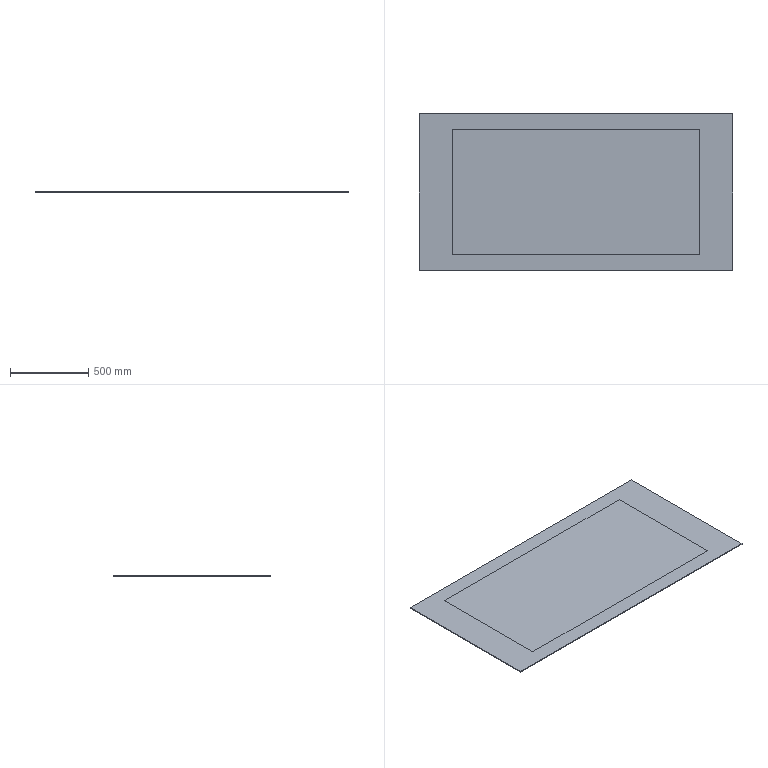Part | SolidWorks | features BaseBody 2 | 2 solids | 12 faces | box 2000 x 1000 x 5 mm | volume 16320000 mm3 | plane 12
STEP:
#1=CARTESIAN_POINT('',(-1000.,-500.,0.));
#2=VERTEX_POINT('',#1);
#3=CARTESIAN_POINT('',(1000.,-500.,0.));
#4=VERTEX_POINT('',#3);
#5=CARTESIAN_POINT('',(0.,-500.,0.));
#6=DIRECTION('',(1.,0.,0.));
#7=VECTOR('',#6,1000.);
#8=LINE('',#5,#7);
#9=EDGE_CURVE('',#2,#4,#8,.T.);
#10=ORIENTED_EDGE('',*,*,#9,.F.);
#11=CARTESIAN_POINT('',(-1000.,500.,0.));
#12=VERTEX_POINT('',#11);
#13=CARTESIAN_POINT('',(-1000.,0.,0.));
#14=DIRECTION('',(0.,-1.,0.));
#15=VECTOR('',#14,1000.);
#16=LINE('',#13,#15);
#17=EDGE_CURVE('',#12,#2,#16,.T.);
#18=ORIENTED_EDGE('',*,*,#17,.F.);
#19=CARTESIAN_POINT('',(1000.,500.,0.));
#20=VERTEX_POINT('',#19);
#21=CARTESIAN_POINT('',(0.,500.,0.));
#22=DIRECTION('',(-1.,0.,0.));
#23=VECTOR('',#22,1000.);
#24=LINE('',#21,#23);
#25=EDGE_CURVE('',#20,#12,#24,.T.);
#26=ORIENTED_EDGE('',*,*,#25,.F.);
#27=CARTESIAN_POINT('',(1000.,0.,0.));
#28=DIRECTION('',(0.,1.,0.));
#29=VECTOR('',#28,1000.);
#30=LINE('',#27,#29);
#31=EDGE_CURVE('',#4,#20,#30,.T.);
#32=ORIENTED_EDGE('',*,*,#31,.F.);
#33=EDGE_LOOP('',(#10,#18,#26,#32));
#34=FACE_OUTER_BOUND('',#33,.T.);
#35=CARTESIAN_POINT('',(0.,0.,0.));
#36=DIRECTION('',(0.,0.,1.));
#37=DIRECTION('',(1.,0.,0.));
#38=AXIS2_PLACEMENT_3D('',#35,#36,#37);
#39=PLANE('',#38);
#40=ADVANCED_FACE('',(#34),#39,.F.);
#41=ORIENTED_EDGE('',*,*,#31,.T.);
#42=CARTESIAN_POINT('',(1000.,500.,5.));
#43=VERTEX_POINT('',#42);
#44=CARTESIAN_POINT('',(1000.,500.,0.));
#45=DIRECTION('',(0.,0.,1.));
#46=VECTOR('',#45,1000.);
#47=LINE('',#44,#46);
#48=EDGE_CURVE('',#20,#43,#47,.T.);
#49=ORIENTED_EDGE('',*,*,#48,.T.);
#50=CARTESIAN_POINT('',(1000.,-500.,5.));
#51=VERTEX_POINT('',#50);
#52=CARTESIAN_POINT('',(1000.,500.,5.));
#53=DIRECTION('',(0.,-1.,0.));
#54=VECTOR('',#53,1000.);
#55=LINE('',#52,#54);
#56=EDGE_CURVE('',#43,#51,#55,.T.);
#57=ORIENTED_EDGE('',*,*,#56,.T.);
#58=CARTESIAN_POINT('',(1000.,-500.,0.));
#59=DIRECTION('',(0.,0.,-1.));
#60=VECTOR('',#59,1000.);
#61=LINE('',#58,#60);
#62=EDGE_CURVE('',#51,#4,#61,.T.);
#63=ORIENTED_EDGE('',*,*,#62,.T.);
#64=EDGE_LOOP('',(#41,#49,#57,#63));
#65=FACE_OUTER_BOUND('',#64,.T.);
#66=CARTESIAN_POINT('',(1000.,500.,0.));
#67=DIRECTION('',(1.,0.,0.));
#68=DIRECTION('',(0.,0.,-1.));
#69=AXIS2_PLACEMENT_3D('',#66,#67,#68);
#70=PLANE('',#69);
#71=ADVANCED_FACE('',(#65),#70,.T.);
#72=ORIENTED_EDGE('',*,*,#9,.T.);
#73=ORIENTED_EDGE('',*,*,#62,.F.);
#74=CARTESIAN_POINT('',(-1000.,-500.,5.));
#75=VERTEX_POINT('',#74);
#76=CARTESIAN_POINT('',(-1000.,-500.,5.));
#77=DIRECTION('',(-1.,0.,0.));
#78=VECTOR('',#77,1000.);
#79=LINE('',#76,#78);
#80=EDGE_CURVE('',#51,#75,#79,.T.);
#81=ORIENTED_EDGE('',*,*,#80,.T.);
#82=CARTESIAN_POINT('',(-1000.,-500.,0.));
#83=DIRECTION('',(0.,0.,-1.));
#84=VECTOR('',#83,1000.);
#85=LINE('',#82,#84);
#86=EDGE_CURVE('',#75,#2,#85,.T.);
#87=ORIENTED_EDGE('',*,*,#86,.T.);
#88=EDGE_LOOP('',(#72,#73,#81,#87));
#89=FACE_OUTER_BOUND('',#88,.T.);
#90=CARTESIAN_POINT('',(-1000.,-500.,0.));
#91=DIRECTION('',(0.,-1.,0.));
#92=DIRECTION('',(0.,0.,-1.));
#93=AXIS2_PLACEMENT_3D('',#90,#91,#92);
#94=PLANE('',#93);
#95=ADVANCED_FACE('',(#89),#94,.T.);
#96=ORIENTED_EDGE('',*,*,#17,.T.);
#97=ORIENTED_EDGE('',*,*,#86,.F.);
#98=CARTESIAN_POINT('',(-1000.,500.,5.));
#99=VERTEX_POINT('',#98);
#100=CARTESIAN_POINT('',(-1000.,500.,5.));
#101=DIRECTION('',(0.,1.,0.));
#102=VECTOR('',#101,1000.);
#103=LINE('',#100,#102);
#104=EDGE_CURVE('',#75,#99,#103,.T.);
#105=ORIENTED_EDGE('',*,*,#104,.T.);
#106=CARTESIAN_POINT('',(-1000.,500.,0.));
#107=DIRECTION('',(0.,0.,-1.));
#108=VECTOR('',#107,1000.);
#109=LINE('',#106,#108);
#110=EDGE_CURVE('',#99,#12,#109,.T.);
#111=ORIENTED_EDGE('',*,*,#110,.T.);
#112=EDGE_LOOP('',(#96,#97,#105,#111));
#113=FACE_OUTER_BOUND('',#112,.T.);
#114=CARTESIAN_POINT('',(-1000.,500.,0.));
#115=DIRECTION('',(-1.,0.,0.));
#116=DIRECTION('',(0.,-1.,0.));
#117=AXIS2_PLACEMENT_3D('',#114,#115,#116);
#118=PLANE('',#117);
#119=ADVANCED_FACE('',(#113),#118,.T.);
#120=ORIENTED_EDGE('',*,*,#25,.T.);
#121=ORIENTED_EDGE('',*,*,#110,.F.);
#122=CARTESIAN_POINT('',(-1000.,500.,5.));
#123=DIRECTION('',(1.,0.,0.));
#124=VECTOR('',#123,1000.);
#125=LINE('',#122,#124);
#126=EDGE_CURVE('',#99,#43,#125,.T.);
#127=ORIENTED_EDGE('',*,*,#126,.T.);
#128=ORIENTED_EDGE('',*,*,#48,.F.);
#129=EDGE_LOOP('',(#120,#121,#127,#128));
#130=FACE_OUTER_BOUND('',#129,.T.);
#131=CARTESIAN_POINT('',(-1000.,500.,0.));
#132=DIRECTION('',(0.,1.,0.));
#133=DIRECTION('',(0.,0.,1.));
#134=AXIS2_PLACEMENT_3D('',#131,#132,#133);
#135=PLANE('',#134);
#136=ADVANCED_FACE('',(#130),#135,.T.);
#137=ORIENTED_EDGE('',*,*,#104,.F.);
#138=ORIENTED_EDGE('',*,*,#80,.F.);
#139=ORIENTED_EDGE('',*,*,#56,.F.);
#140=ORIENTED_EDGE('',*,*,#126,.F.);
#141=EDGE_LOOP('',(#137,#138,#139,#140));
#142=FACE_OUTER_BOUND('',#141,.T.);
#143=CARTESIAN_POINT('',(0.,0.,5.));
#144=DIRECTION('',(0.,0.,1.));
#145=DIRECTION('',(1.,0.,0.));
#146=AXIS2_PLACEMENT_3D('',#143,#144,#145);
#147=PLANE('',#146);
#148=ADVANCED_FACE('',(#142),#147,.T.);
#149=CLOSED_SHELL('',(#40,#71,#95,#119,#136,#148));
#150=MANIFOLD_SOLID_BREP('',#149);
#151=CARTESIAN_POINT('',(-790.,400.,5.));
#152=VERTEX_POINT('',#151);
#153=CARTESIAN_POINT('',(-790.,-400.,5.));
#154=VERTEX_POINT('',#153);
#155=CARTESIAN_POINT('',(-790.,0.,5.));
#156=DIRECTION('',(0.,-1.,0.));
#157=VECTOR('',#156,1000.);
#158=LINE('',#155,#157);
#159=EDGE_CURVE('',#152,#154,#158,.T.);
#160=ORIENTED_EDGE('',*,*,#159,.T.);
#161=CARTESIAN_POINT('',(790.,-400.,5.));
#162=VERTEX_POINT('',#161);
#163=CARTESIAN_POINT('',(0.,-400.,5.));
#164=DIRECTION('',(1.,0.,0.));
#165=VECTOR('',#164,1000.);
#166=LINE('',#163,#165);
#167=EDGE_CURVE('',#154,#162,#166,.T.);
#168=ORIENTED_EDGE('',*,*,#167,.T.);
#169=CARTESIAN_POINT('',(790.,400.,5.));
#170=VERTEX_POINT('',#169);
#171=CARTESIAN_POINT('',(790.,0.,5.));
#172=DIRECTION('',(0.,1.,0.));
#173=VECTOR('',#172,1000.);
#174=LINE('',#171,#173);
#175=EDGE_CURVE('',#162,#170,#174,.T.);
#176=ORIENTED_EDGE('',*,*,#175,.T.);
#177=CARTESIAN_POINT('',(0.,400.,5.));
#178=DIRECTION('',(-1.,0.,0.));
#179=VECTOR('',#178,1000.);
#180=LINE('',#177,#179);
#181=EDGE_CURVE('',#170,#152,#180,.T.);
#182=ORIENTED_EDGE('',*,*,#181,.T.);
#183=EDGE_LOOP('',(#160,#168,#176,#182));
#184=FACE_OUTER_BOUND('',#183,.T.);
#185=CARTESIAN_POINT('',(0.,0.,5.));
#186=DIRECTION('',(0.,0.,1.));
#187=DIRECTION('',(1.,0.,0.));
#188=AXIS2_PLACEMENT_3D('',#185,#186,#187);
#189=PLANE('',#188);
#190=ADVANCED_FACE('',(#184),#189,.T.);
#191=CARTESIAN_POINT('',(790.,-400.,0.));
#192=VERTEX_POINT('',#191);
#193=CARTESIAN_POINT('',(790.,-400.,5.));
#194=DIRECTION('',(0.,0.,-1.));
#195=VECTOR('',#194,1000.);
#196=LINE('',#193,#195);
#197=EDGE_CURVE('',#162,#192,#196,.T.);
#198=ORIENTED_EDGE('',*,*,#197,.F.);
#199=ORIENTED_EDGE('',*,*,#167,.F.);
#200=CARTESIAN_POINT('',(-790.,-400.,0.));
#201=VERTEX_POINT('',#200);
#202=CARTESIAN_POINT('',(-790.,-400.,5.));
#203=DIRECTION('',(0.,0.,1.));
#204=VECTOR('',#203,1000.);
#205=LINE('',#202,#204);
#206=EDGE_CURVE('',#201,#154,#205,.T.);
#207=ORIENTED_EDGE('',*,*,#206,.F.);
#208=CARTESIAN_POINT('',(-790.,-400.,0.));
#209=DIRECTION('',(-1.,0.,0.));
#210=VECTOR('',#209,1000.);
#211=LINE('',#208,#210);
#212=EDGE_CURVE('',#192,#201,#211,.T.);
#213=ORIENTED_EDGE('',*,*,#212,.F.);
#214=EDGE_LOOP('',(#198,#199,#207,#213));
#215=FACE_OUTER_BOUND('',#214,.T.);
#216=CARTESIAN_POINT('',(-790.,-400.,5.));
#217=DIRECTION('',(0.,1.,0.));
#218=DIRECTION('',(0.,0.,1.));
#219=AXIS2_PLACEMENT_3D('',#216,#217,#218);
#220=PLANE('',#219);
#221=ADVANCED_FACE('',(#215),#220,.F.);
#222=ORIENTED_EDGE('',*,*,#206,.T.);
#223=ORIENTED_EDGE('',*,*,#159,.F.);
#224=CARTESIAN_POINT('',(-790.,400.,0.));
#225=VERTEX_POINT('',#224);
#226=CARTESIAN_POINT('',(-790.,400.,5.));
#227=DIRECTION('',(0.,0.,1.));
#228=VECTOR('',#227,1000.);
#229=LINE('',#226,#228);
#230=EDGE_CURVE('',#225,#152,#229,.T.);
#231=ORIENTED_EDGE('',*,*,#230,.F.);
#232=CARTESIAN_POINT('',(-790.,400.,0.));
#233=DIRECTION('',(0.,1.,0.));
#234=VECTOR('',#233,1000.);
#235=LINE('',#232,#234);
#236=EDGE_CURVE('',#201,#225,#235,.T.);
#237=ORIENTED_EDGE('',*,*,#236,.F.);
#238=EDGE_LOOP('',(#222,#223,#231,#237));
#239=FACE_OUTER_BOUND('',#238,.T.);
#240=CARTESIAN_POINT('',(-790.,400.,5.));
#241=DIRECTION('',(1.,0.,0.));
#242=DIRECTION('',(0.,0.,-1.));
#243=AXIS2_PLACEMENT_3D('',#240,#241,#242);
#244=PLANE('',#243);
#245=ADVANCED_FACE('',(#239),#244,.F.);
#246=ORIENTED_EDGE('',*,*,#230,.T.);
#247=ORIENTED_EDGE('',*,*,#181,.F.);
#248=CARTESIAN_POINT('',(790.,400.,0.));
#249=VERTEX_POINT('',#248);
#250=CARTESIAN_POINT('',(790.,400.,5.));
#251=DIRECTION('',(0.,0.,1.));
#252=VECTOR('',#251,1000.);
#253=LINE('',#250,#252);
#254=EDGE_CURVE('',#249,#170,#253,.T.);
#255=ORIENTED_EDGE('',*,*,#254,.F.);
#256=CARTESIAN_POINT('',(-790.,400.,0.));
#257=DIRECTION('',(1.,0.,0.));
#258=VECTOR('',#257,1000.);
#259=LINE('',#256,#258);
#260=EDGE_CURVE('',#225,#249,#259,.T.);
#261=ORIENTED_EDGE('',*,*,#260,.F.);
#262=EDGE_LOOP('',(#246,#247,#255,#261));
#263=FACE_OUTER_BOUND('',#262,.T.);
#264=CARTESIAN_POINT('',(-790.,400.,5.));
#265=DIRECTION('',(0.,-1.,0.));
#266=DIRECTION('',(0.,0.,-1.));
#267=AXIS2_PLACEMENT_3D('',#264,#265,#266);
#268=PLANE('',#267);
#269=ADVANCED_FACE('',(#263),#268,.F.);
#270=ORIENTED_EDGE('',*,*,#254,.T.);
#271=ORIENTED_EDGE('',*,*,#175,.F.);
#272=ORIENTED_EDGE('',*,*,#197,.T.);
#273=CARTESIAN_POINT('',(790.,400.,0.));
#274=DIRECTION('',(0.,-1.,0.));
#275=VECTOR('',#274,1000.);
#276=LINE('',#273,#275);
#277=EDGE_CURVE('',#249,#192,#276,.T.);
#278=ORIENTED_EDGE('',*,*,#277,.F.);
#279=EDGE_LOOP('',(#270,#271,#272,#278));
#280=FACE_OUTER_BOUND('',#279,.T.);
#281=CARTESIAN_POINT('',(790.,400.,5.));
#282=DIRECTION('',(-1.,0.,0.));
#283=DIRECTION('',(0.,0.,1.));
#284=AXIS2_PLACEMENT_3D('',#281,#282,#283);
#285=PLANE('',#284);
#286=ADVANCED_FACE('',(#280),#285,.F.);
#287=ORIENTED_EDGE('',*,*,#212,.T.);
#288=ORIENTED_EDGE('',*,*,#236,.T.);
#289=ORIENTED_EDGE('',*,*,#260,.T.);
#290=ORIENTED_EDGE('',*,*,#277,.T.);
#291=EDGE_LOOP('',(#287,#288,#289,#290));
#292=FACE_OUTER_BOUND('',#291,.T.);
#293=CARTESIAN_POINT('',(0.,0.,0.));
#294=DIRECTION('',(0.,0.,1.));
#295=DIRECTION('',(1.,0.,0.));
#296=AXIS2_PLACEMENT_3D('',#293,#294,#295);
#297=PLANE('',#296);
#298=ADVANCED_FACE('',(#292),#297,.F.);
#299=CLOSED_SHELL('',(#190,#221,#245,#269,#286,#298));
#300=MANIFOLD_SOLID_BREP('',#299);
#301=CARTESIAN_POINT('',(0.,0.,0.));
#302=DIRECTION('',(0.,0.,1.));
#303=DIRECTION('',(1.,0.,0.));
#304=AXIS2_PLACEMENT_3D('',#301,#302,#303);
#305=(LENGTH_UNIT()NAMED_UNIT(*)SI_UNIT(.MILLI.,.METRE.));
#306=UNCERTAINTY_MEASURE_WITH_UNIT(LENGTH_MEASURE(0.00001),#305,'','');
#307=(NAMED_UNIT(*)PLANE_ANGLE_UNIT()SI_UNIT($,.RADIAN.));
#308=(NAMED_UNIT(*)SI_UNIT($,.STERADIAN.)SOLID_ANGLE_UNIT());
#309=(GEOMETRIC_REPRESENTATION_CONTEXT(3)GLOBAL_UNCERTAINTY_ASSIGNED_CONTEXT((#306))GLOBAL_UNIT_ASSIGNED_CONTEXT((#305,#307,#308))REPRESENTATION_CONTEXT('',''));
#310=ADVANCED_BREP_SHAPE_REPRESENTATION('',(#150,#300,#304),#309);